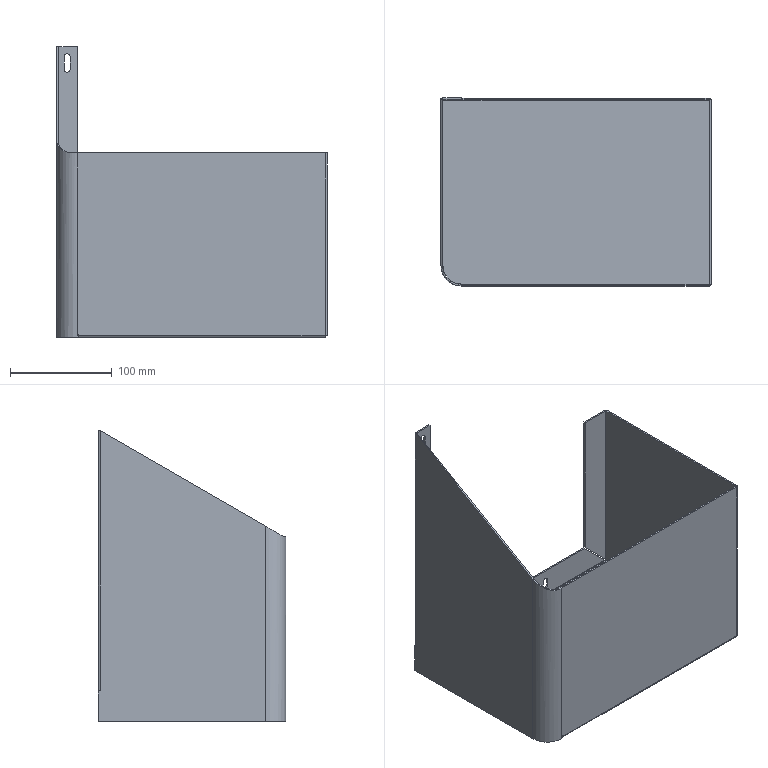Part | SolidWorks | features ICE 5, EdgeFlange 2, SMBaseFlange 2, FlatPattern 1, SMMiteredFlange 1, SheetMetal 1 | 1 solid | 79 faces | box 265 x 184 x 285 mm | volume 277384 mm3 | plane 52 | cylinder 22 | spline 5 | commonest cylinder face diameters 6 x9 1 x5 4 x5 36 x1 37 x1 40 x1